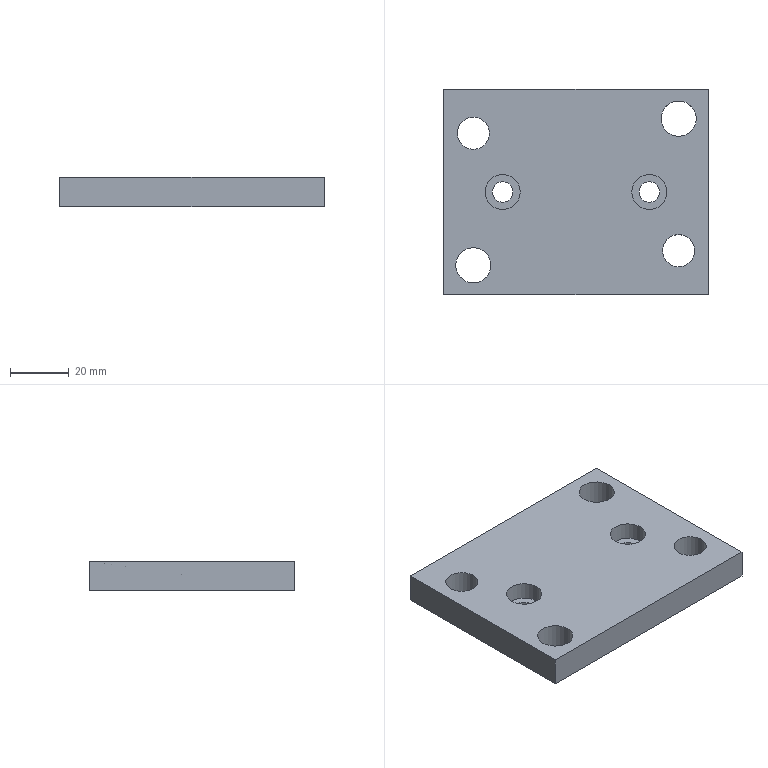Part | NX | features solid 2 | 1 solid | 16 faces | box 90 x 70 x 10 mm | volume 57172 mm3 | plane 8 | cylinder 8 | commonest cylinder face diameters 12 x4 7 x2 11 x2
STEP:
#1=CARTESIAN_POINT('',(594.,70.,60.));
#2=VERTEX_POINT('',#1);
#3=CARTESIAN_POINT('',(600.,70.,60.));
#4=DIRECTION('',(0.,0.,-1.));
#5=DIRECTION('',(-1.,0.,0.));
#6=AXIS2_PLACEMENT_3D('',#3,#4,#5);
#7=CIRCLE('',#6,6.);
#8=EDGE_CURVE('',#2,#2,#7,.F.);
#9=ORIENTED_EDGE('',*,*,#8,.F.);
#10=EDGE_LOOP('',(#9));
#11=FACE_BOUND('',#10,.T.);
#12=CARTESIAN_POINT('',(524.,20.,60.));
#13=VERTEX_POINT('',#12);
#14=CARTESIAN_POINT('',(530.,20.,60.));
#15=DIRECTION('',(0.,0.,-1.));
#16=DIRECTION('',(-1.,0.,0.));
#17=AXIS2_PLACEMENT_3D('',#14,#15,#16);
#18=CIRCLE('',#17,6.);
#19=EDGE_CURVE('',#13,#13,#18,.F.);
#20=ORIENTED_EDGE('',*,*,#19,.F.);
#21=EDGE_LOOP('',(#20));
#22=FACE_BOUND('',#21,.T.);
#23=CARTESIAN_POINT('',(584.,45.,60.));
#24=VERTEX_POINT('',#23);
#25=CARTESIAN_POINT('',(590.,45.,60.));
#26=DIRECTION('',(0.,0.,-1.));
#27=DIRECTION('',(-1.,0.,0.));
#28=AXIS2_PLACEMENT_3D('',#25,#26,#27);
#29=CIRCLE('',#28,6.);
#30=EDGE_CURVE('',#24,#24,#29,.T.);
#31=ORIENTED_EDGE('',*,*,#30,.T.);
#32=EDGE_LOOP('',(#31));
#33=FACE_BOUND('',#32,.T.);
#34=CARTESIAN_POINT('',(534.,45.,60.));
#35=VERTEX_POINT('',#34);
#36=CARTESIAN_POINT('',(540.,45.,60.));
#37=DIRECTION('',(0.,0.,-1.));
#38=DIRECTION('',(-1.,0.,0.));
#39=AXIS2_PLACEMENT_3D('',#36,#37,#38);
#40=CIRCLE('',#39,6.);
#41=EDGE_CURVE('',#35,#35,#40,.T.);
#42=ORIENTED_EDGE('',*,*,#41,.T.);
#43=EDGE_LOOP('',(#42));
#44=FACE_BOUND('',#43,.T.);
#45=CARTESIAN_POINT('',(610.,10.,60.));
#46=VERTEX_POINT('',#45);
#47=CARTESIAN_POINT('',(520.,10.,60.));
#48=VERTEX_POINT('',#47);
#49=CARTESIAN_POINT('',(610.,10.,60.));
#50=DIRECTION('',(-1.,0.,0.));
#51=VECTOR('',#50,1000.);
#52=LINE('',#49,#51);
#53=EDGE_CURVE('',#46,#48,#52,.T.);
#54=ORIENTED_EDGE('',*,*,#53,.F.);
#55=CARTESIAN_POINT('',(610.,80.,60.));
#56=VERTEX_POINT('',#55);
#57=CARTESIAN_POINT('',(610.,80.,60.));
#58=DIRECTION('',(0.,-1.,0.));
#59=VECTOR('',#58,1000.);
#60=LINE('',#57,#59);
#61=EDGE_CURVE('',#56,#46,#60,.T.);
#62=ORIENTED_EDGE('',*,*,#61,.F.);
#63=CARTESIAN_POINT('',(520.,80.,60.));
#64=VERTEX_POINT('',#63);
#65=CARTESIAN_POINT('',(520.,80.,60.));
#66=DIRECTION('',(1.,0.,0.));
#67=VECTOR('',#66,1000.);
#68=LINE('',#65,#67);
#69=EDGE_CURVE('',#64,#56,#68,.T.);
#70=ORIENTED_EDGE('',*,*,#69,.F.);
#71=CARTESIAN_POINT('',(520.,10.,60.));
#72=DIRECTION('',(0.,1.,0.));
#73=VECTOR('',#72,1000.);
#74=LINE('',#71,#73);
#75=EDGE_CURVE('',#48,#64,#74,.T.);
#76=ORIENTED_EDGE('',*,*,#75,.F.);
#77=EDGE_LOOP('',(#54,#62,#70,#76));
#78=FACE_BOUND('',#77,.T.);
#79=CARTESIAN_POINT('',(594.5,25.,60.));
#80=VERTEX_POINT('',#79);
#81=CARTESIAN_POINT('',(600.,25.,60.));
#82=DIRECTION('',(0.,0.,-1.));
#83=DIRECTION('',(-1.,0.,0.));
#84=AXIS2_PLACEMENT_3D('',#81,#82,#83);
#85=CIRCLE('',#84,5.5);
#86=EDGE_CURVE('',#80,#80,#85,.F.);
#87=ORIENTED_EDGE('',*,*,#86,.F.);
#88=EDGE_LOOP('',(#87));
#89=FACE_BOUND('',#88,.T.);
#90=CARTESIAN_POINT('',(524.5,65.,60.));
#91=VERTEX_POINT('',#90);
#92=CARTESIAN_POINT('',(530.,65.,60.));
#93=DIRECTION('',(0.,0.,-1.));
#94=DIRECTION('',(-1.,0.,0.));
#95=AXIS2_PLACEMENT_3D('',#92,#93,#94);
#96=CIRCLE('',#95,5.5);
#97=EDGE_CURVE('',#91,#91,#96,.F.);
#98=ORIENTED_EDGE('',*,*,#97,.F.);
#99=EDGE_LOOP('',(#98));
#100=FACE_BOUND('',#99,.T.);
#101=CARTESIAN_POINT('',(520.,10.,60.));
#102=DIRECTION('',(0.,0.,-1.));
#103=DIRECTION('',(-1.,0.,0.));
#104=AXIS2_PLACEMENT_3D('',#101,#102,#103);
#105=PLANE('',#104);
#106=ADVANCED_FACE('',(#11,#22,#33,#44,#78,#89,#100),#105,.F.);
#107=CARTESIAN_POINT('',(594.,70.,50.));
#108=VERTEX_POINT('',#107);
#109=CARTESIAN_POINT('',(600.,70.,50.));
#110=DIRECTION('',(0.,0.,-1.));
#111=DIRECTION('',(-1.,0.,0.));
#112=AXIS2_PLACEMENT_3D('',#109,#110,#111);
#113=CIRCLE('',#112,6.);
#114=EDGE_CURVE('',#108,#108,#113,.T.);
#115=ORIENTED_EDGE('',*,*,#114,.F.);
#116=EDGE_LOOP('',(#115));
#117=FACE_BOUND('',#116,.T.);
#118=CARTESIAN_POINT('',(524.,20.,50.));
#119=VERTEX_POINT('',#118);
#120=CARTESIAN_POINT('',(530.,20.,50.));
#121=DIRECTION('',(0.,0.,-1.));
#122=DIRECTION('',(-1.,0.,0.));
#123=AXIS2_PLACEMENT_3D('',#120,#121,#122);
#124=CIRCLE('',#123,6.);
#125=EDGE_CURVE('',#119,#119,#124,.T.);
#126=ORIENTED_EDGE('',*,*,#125,.F.);
#127=EDGE_LOOP('',(#126));
#128=FACE_BOUND('',#127,.T.);
#129=CARTESIAN_POINT('',(586.5,45.,50.));
#130=VERTEX_POINT('',#129);
#131=CARTESIAN_POINT('',(590.,45.,50.));
#132=DIRECTION('',(0.,0.,-1.));
#133=DIRECTION('',(-1.,0.,0.));
#134=AXIS2_PLACEMENT_3D('',#131,#132,#133);
#135=CIRCLE('',#134,3.5);
#136=EDGE_CURVE('',#130,#130,#135,.T.);
#137=ORIENTED_EDGE('',*,*,#136,.F.);
#138=EDGE_LOOP('',(#137));
#139=FACE_BOUND('',#138,.T.);
#140=CARTESIAN_POINT('',(536.5,45.,50.));
#141=VERTEX_POINT('',#140);
#142=CARTESIAN_POINT('',(540.,45.,50.));
#143=DIRECTION('',(0.,0.,-1.));
#144=DIRECTION('',(-1.,0.,0.));
#145=AXIS2_PLACEMENT_3D('',#142,#143,#144);
#146=CIRCLE('',#145,3.5);
#147=EDGE_CURVE('',#141,#141,#146,.T.);
#148=ORIENTED_EDGE('',*,*,#147,.F.);
#149=EDGE_LOOP('',(#148));
#150=FACE_BOUND('',#149,.T.);
#151=CARTESIAN_POINT('',(610.,10.,50.));
#152=VERTEX_POINT('',#151);
#153=CARTESIAN_POINT('',(520.,10.,50.));
#154=VERTEX_POINT('',#153);
#155=CARTESIAN_POINT('',(610.,10.,50.));
#156=DIRECTION('',(-1.,0.,0.));
#157=VECTOR('',#156,1000.);
#158=LINE('',#155,#157);
#159=EDGE_CURVE('',#152,#154,#158,.T.);
#160=ORIENTED_EDGE('',*,*,#159,.T.);
#161=CARTESIAN_POINT('',(520.,80.,50.));
#162=VERTEX_POINT('',#161);
#163=CARTESIAN_POINT('',(520.,10.,50.));
#164=DIRECTION('',(0.,1.,0.));
#165=VECTOR('',#164,1000.);
#166=LINE('',#163,#165);
#167=EDGE_CURVE('',#154,#162,#166,.T.);
#168=ORIENTED_EDGE('',*,*,#167,.T.);
#169=CARTESIAN_POINT('',(610.,80.,50.));
#170=VERTEX_POINT('',#169);
#171=CARTESIAN_POINT('',(520.,80.,50.));
#172=DIRECTION('',(1.,0.,0.));
#173=VECTOR('',#172,1000.);
#174=LINE('',#171,#173);
#175=EDGE_CURVE('',#162,#170,#174,.T.);
#176=ORIENTED_EDGE('',*,*,#175,.T.);
#177=CARTESIAN_POINT('',(610.,80.,50.));
#178=DIRECTION('',(0.,-1.,0.));
#179=VECTOR('',#178,1000.);
#180=LINE('',#177,#179);
#181=EDGE_CURVE('',#170,#152,#180,.T.);
#182=ORIENTED_EDGE('',*,*,#181,.T.);
#183=EDGE_LOOP('',(#160,#168,#176,#182));
#184=FACE_BOUND('',#183,.T.);
#185=CARTESIAN_POINT('',(594.5,25.,50.));
#186=VERTEX_POINT('',#185);
#187=CARTESIAN_POINT('',(600.,25.,50.));
#188=DIRECTION('',(0.,0.,-1.));
#189=DIRECTION('',(-1.,0.,0.));
#190=AXIS2_PLACEMENT_3D('',#187,#188,#189);
#191=CIRCLE('',#190,5.5);
#192=EDGE_CURVE('',#186,#186,#191,.T.);
#193=ORIENTED_EDGE('',*,*,#192,.F.);
#194=EDGE_LOOP('',(#193));
#195=FACE_BOUND('',#194,.T.);
#196=CARTESIAN_POINT('',(524.5,65.,50.));
#197=VERTEX_POINT('',#196);
#198=CARTESIAN_POINT('',(530.,65.,50.));
#199=DIRECTION('',(0.,0.,-1.));
#200=DIRECTION('',(-1.,0.,0.));
#201=AXIS2_PLACEMENT_3D('',#198,#199,#200);
#202=CIRCLE('',#201,5.5);
#203=EDGE_CURVE('',#197,#197,#202,.T.);
#204=ORIENTED_EDGE('',*,*,#203,.F.);
#205=EDGE_LOOP('',(#204));
#206=FACE_BOUND('',#205,.T.);
#207=CARTESIAN_POINT('',(520.,10.,50.));
#208=DIRECTION('',(0.,0.,-1.));
#209=DIRECTION('',(-1.,0.,0.));
#210=AXIS2_PLACEMENT_3D('',#207,#208,#209);
#211=PLANE('',#210);
#212=ADVANCED_FACE('',(#117,#128,#139,#150,#184,#195,#206),#211,.T.);
#213=ORIENTED_EDGE('',*,*,#159,.F.);
#214=CARTESIAN_POINT('',(610.,10.,60.));
#215=DIRECTION('',(0.,0.,-1.));
#216=VECTOR('',#215,1000.);
#217=LINE('',#214,#216);
#218=EDGE_CURVE('',#46,#152,#217,.T.);
#219=ORIENTED_EDGE('',*,*,#218,.F.);
#220=ORIENTED_EDGE('',*,*,#53,.T.);
#221=CARTESIAN_POINT('',(520.,10.,60.));
#222=DIRECTION('',(0.,0.,-1.));
#223=VECTOR('',#222,1000.);
#224=LINE('',#221,#223);
#225=EDGE_CURVE('',#48,#154,#224,.T.);
#226=ORIENTED_EDGE('',*,*,#225,.T.);
#227=EDGE_LOOP('',(#213,#219,#220,#226));
#228=FACE_BOUND('',#227,.T.);
#229=CARTESIAN_POINT('',(610.,10.,60.));
#230=DIRECTION('',(0.,-1.,0.));
#231=DIRECTION('',(0.,0.,-1.));
#232=AXIS2_PLACEMENT_3D('',#229,#230,#231);
#233=PLANE('',#232);
#234=ADVANCED_FACE('',(#228),#233,.T.);
#235=ORIENTED_EDGE('',*,*,#167,.F.);
#236=ORIENTED_EDGE('',*,*,#225,.F.);
#237=ORIENTED_EDGE('',*,*,#75,.T.);
#238=CARTESIAN_POINT('',(520.,80.,60.));
#239=DIRECTION('',(0.,0.,-1.));
#240=VECTOR('',#239,1000.);
#241=LINE('',#238,#240);
#242=EDGE_CURVE('',#64,#162,#241,.T.);
#243=ORIENTED_EDGE('',*,*,#242,.T.);
#244=EDGE_LOOP('',(#235,#236,#237,#243));
#245=FACE_BOUND('',#244,.T.);
#246=CARTESIAN_POINT('',(520.,10.,60.));
#247=DIRECTION('',(-1.,0.,0.));
#248=DIRECTION('',(0.,0.,1.));
#249=AXIS2_PLACEMENT_3D('',#246,#247,#248);
#250=PLANE('',#249);
#251=ADVANCED_FACE('',(#245),#250,.T.);
#252=ORIENTED_EDGE('',*,*,#175,.F.);
#253=ORIENTED_EDGE('',*,*,#242,.F.);
#254=ORIENTED_EDGE('',*,*,#69,.T.);
#255=CARTESIAN_POINT('',(610.,80.,60.));
#256=DIRECTION('',(0.,0.,-1.));
#257=VECTOR('',#256,1000.);
#258=LINE('',#255,#257);
#259=EDGE_CURVE('',#56,#170,#258,.T.);
#260=ORIENTED_EDGE('',*,*,#259,.T.);
#261=EDGE_LOOP('',(#252,#253,#254,#260));
#262=FACE_BOUND('',#261,.T.);
#263=CARTESIAN_POINT('',(520.,80.,60.));
#264=DIRECTION('',(0.,1.,0.));
#265=DIRECTION('',(0.,0.,1.));
#266=AXIS2_PLACEMENT_3D('',#263,#264,#265);
#267=PLANE('',#266);
#268=ADVANCED_FACE('',(#262),#267,.T.);
#269=ORIENTED_EDGE('',*,*,#181,.F.);
#270=ORIENTED_EDGE('',*,*,#259,.F.);
#271=ORIENTED_EDGE('',*,*,#61,.T.);
#272=ORIENTED_EDGE('',*,*,#218,.T.);
#273=EDGE_LOOP('',(#269,#270,#271,#272));
#274=FACE_BOUND('',#273,.T.);
#275=CARTESIAN_POINT('',(610.,80.,60.));
#276=DIRECTION('',(1.,0.,0.));
#277=DIRECTION('',(0.,0.,-1.));
#278=AXIS2_PLACEMENT_3D('',#275,#276,#277);
#279=PLANE('',#278);
#280=ADVANCED_FACE('',(#274),#279,.T.);
#281=ORIENTED_EDGE('',*,*,#147,.T.);
#282=EDGE_LOOP('',(#281));
#283=FACE_BOUND('',#282,.T.);
#284=CARTESIAN_POINT('',(536.5,45.,54.));
#285=VERTEX_POINT('',#284);
#286=CARTESIAN_POINT('',(540.,45.,54.));
#287=DIRECTION('',(0.,0.,-1.));
#288=DIRECTION('',(-1.,0.,0.));
#289=AXIS2_PLACEMENT_3D('',#286,#287,#288);
#290=CIRCLE('',#289,3.5);
#291=EDGE_CURVE('',#285,#285,#290,.T.);
#292=ORIENTED_EDGE('',*,*,#291,.F.);
#293=EDGE_LOOP('',(#292));
#294=FACE_BOUND('',#293,.T.);
#295=CARTESIAN_POINT('',(540.,45.,10.));
#296=DIRECTION('',(0.,0.,-1.));
#297=DIRECTION('',(-1.,0.,0.));
#298=AXIS2_PLACEMENT_3D('',#295,#296,#297);
#299=CYLINDRICAL_SURFACE('',#298,3.5);
#300=ADVANCED_FACE('',(#283,#294),#299,.F.);
#301=ORIENTED_EDGE('',*,*,#291,.T.);
#302=EDGE_LOOP('',(#301));
#303=FACE_BOUND('',#302,.T.);
#304=CARTESIAN_POINT('',(534.,45.,54.));
#305=VERTEX_POINT('',#304);
#306=CARTESIAN_POINT('',(540.,45.,54.));
#307=DIRECTION('',(0.,0.,-1.));
#308=DIRECTION('',(-1.,0.,0.));
#309=AXIS2_PLACEMENT_3D('',#306,#307,#308);
#310=CIRCLE('',#309,6.);
#311=EDGE_CURVE('',#305,#305,#310,.T.);
#312=ORIENTED_EDGE('',*,*,#311,.F.);
#313=EDGE_LOOP('',(#312));
#314=FACE_BOUND('',#313,.T.);
#315=CARTESIAN_POINT('',(540.,45.,54.));
#316=DIRECTION('',(0.,0.,-1.));
#317=DIRECTION('',(-1.,0.,0.));
#318=AXIS2_PLACEMENT_3D('',#315,#316,#317);
#319=PLANE('',#318);
#320=ADVANCED_FACE('',(#303,#314),#319,.F.);
#321=ORIENTED_EDGE('',*,*,#311,.T.);
#322=EDGE_LOOP('',(#321));
#323=FACE_BOUND('',#322,.T.);
#324=ORIENTED_EDGE('',*,*,#41,.F.);
#325=EDGE_LOOP('',(#324));
#326=FACE_BOUND('',#325,.T.);
#327=CARTESIAN_POINT('',(540.,45.,60.));
#328=DIRECTION('',(0.,0.,-1.));
#329=DIRECTION('',(-1.,0.,0.));
#330=AXIS2_PLACEMENT_3D('',#327,#328,#329);
#331=CYLINDRICAL_SURFACE('',#330,6.);
#332=ADVANCED_FACE('',(#323,#326),#331,.F.);
#333=ORIENTED_EDGE('',*,*,#136,.T.);
#334=EDGE_LOOP('',(#333));
#335=FACE_BOUND('',#334,.T.);
#336=CARTESIAN_POINT('',(586.5,45.,54.));
#337=VERTEX_POINT('',#336);
#338=CARTESIAN_POINT('',(590.,45.,54.));
#339=DIRECTION('',(0.,0.,-1.));
#340=DIRECTION('',(-1.,0.,0.));
#341=AXIS2_PLACEMENT_3D('',#338,#339,#340);
#342=CIRCLE('',#341,3.5);
#343=EDGE_CURVE('',#337,#337,#342,.T.);
#344=ORIENTED_EDGE('',*,*,#343,.F.);
#345=EDGE_LOOP('',(#344));
#346=FACE_BOUND('',#345,.T.);
#347=CARTESIAN_POINT('',(590.,45.,10.));
#348=DIRECTION('',(0.,0.,-1.));
#349=DIRECTION('',(-1.,0.,0.));
#350=AXIS2_PLACEMENT_3D('',#347,#348,#349);
#351=CYLINDRICAL_SURFACE('',#350,3.5);
#352=ADVANCED_FACE('',(#335,#346),#351,.F.);
#353=ORIENTED_EDGE('',*,*,#343,.T.);
#354=EDGE_LOOP('',(#353));
#355=FACE_BOUND('',#354,.T.);
#356=CARTESIAN_POINT('',(584.,45.,54.));
#357=VERTEX_POINT('',#356);
#358=CARTESIAN_POINT('',(590.,45.,54.));
#359=DIRECTION('',(0.,0.,-1.));
#360=DIRECTION('',(-1.,0.,0.));
#361=AXIS2_PLACEMENT_3D('',#358,#359,#360);
#362=CIRCLE('',#361,6.);
#363=EDGE_CURVE('',#357,#357,#362,.T.);
#364=ORIENTED_EDGE('',*,*,#363,.F.);
#365=EDGE_LOOP('',(#364));
#366=FACE_BOUND('',#365,.T.);
#367=CARTESIAN_POINT('',(590.,45.,54.));
#368=DIRECTION('',(0.,0.,-1.));
#369=DIRECTION('',(-1.,0.,0.));
#370=AXIS2_PLACEMENT_3D('',#367,#368,#369);
#371=PLANE('',#370);
#372=ADVANCED_FACE('',(#355,#366),#371,.F.);
#373=ORIENTED_EDGE('',*,*,#363,.T.);
#374=EDGE_LOOP('',(#373));
#375=FACE_BOUND('',#374,.T.);
#376=ORIENTED_EDGE('',*,*,#30,.F.);
#377=EDGE_LOOP('',(#376));
#378=FACE_BOUND('',#377,.T.);
#379=CARTESIAN_POINT('',(590.,45.,60.));
#380=DIRECTION('',(0.,0.,-1.));
#381=DIRECTION('',(-1.,0.,0.));
#382=AXIS2_PLACEMENT_3D('',#379,#380,#381);
#383=CYLINDRICAL_SURFACE('',#382,6.);
#384=ADVANCED_FACE('',(#375,#378),#383,.F.);
#385=ORIENTED_EDGE('',*,*,#125,.T.);
#386=EDGE_LOOP('',(#385));
#387=FACE_BOUND('',#386,.T.);
#388=ORIENTED_EDGE('',*,*,#19,.T.);
#389=EDGE_LOOP('',(#388));
#390=FACE_BOUND('',#389,.T.);
#391=CARTESIAN_POINT('',(530.,20.,50.));
#392=DIRECTION('',(0.,0.,1.));
#393=DIRECTION('',(1.,0.,0.));
#394=AXIS2_PLACEMENT_3D('',#391,#392,#393);
#395=CYLINDRICAL_SURFACE('',#394,6.);
#396=ADVANCED_FACE('',(#387,#390),#395,.F.);
#397=ORIENTED_EDGE('',*,*,#192,.T.);
#398=EDGE_LOOP('',(#397));
#399=FACE_BOUND('',#398,.T.);
#400=ORIENTED_EDGE('',*,*,#86,.T.);
#401=EDGE_LOOP('',(#400));
#402=FACE_BOUND('',#401,.T.);
#403=CARTESIAN_POINT('',(600.,25.,50.));
#404=DIRECTION('',(0.,0.,1.));
#405=DIRECTION('',(1.,0.,0.));
#406=AXIS2_PLACEMENT_3D('',#403,#404,#405);
#407=CYLINDRICAL_SURFACE('',#406,5.5);
#408=ADVANCED_FACE('',(#399,#402),#407,.F.);
#409=ORIENTED_EDGE('',*,*,#114,.T.);
#410=EDGE_LOOP('',(#409));
#411=FACE_BOUND('',#410,.T.);
#412=ORIENTED_EDGE('',*,*,#8,.T.);
#413=EDGE_LOOP('',(#412));
#414=FACE_BOUND('',#413,.T.);
#415=CARTESIAN_POINT('',(600.,70.,50.));
#416=DIRECTION('',(0.,0.,1.));
#417=DIRECTION('',(1.,0.,0.));
#418=AXIS2_PLACEMENT_3D('',#415,#416,#417);
#419=CYLINDRICAL_SURFACE('',#418,6.);
#420=ADVANCED_FACE('',(#411,#414),#419,.F.);
#421=ORIENTED_EDGE('',*,*,#203,.T.);
#422=EDGE_LOOP('',(#421));
#423=FACE_BOUND('',#422,.T.);
#424=ORIENTED_EDGE('',*,*,#97,.T.);
#425=EDGE_LOOP('',(#424));
#426=FACE_BOUND('',#425,.T.);
#427=CARTESIAN_POINT('',(530.,65.,50.));
#428=DIRECTION('',(0.,0.,1.));
#429=DIRECTION('',(1.,0.,0.));
#430=AXIS2_PLACEMENT_3D('',#427,#428,#429);
#431=CYLINDRICAL_SURFACE('',#430,5.5);
#432=ADVANCED_FACE('',(#423,#426),#431,.F.);
#433=CLOSED_SHELL('',(#106,#212,#234,#251,#268,#280,#300,#320,#332,#352,#372,#384,#396,#408,#420,#432));
#434=MANIFOLD_SOLID_BREP('',#433);
#435=(LENGTH_UNIT()NAMED_UNIT(*)SI_UNIT(.MILLI.,.METRE.));
#436=UNCERTAINTY_MEASURE_WITH_UNIT(LENGTH_MEASURE(0.00001),#435,'','');
#437=(NAMED_UNIT(*)PLANE_ANGLE_UNIT()SI_UNIT($,.RADIAN.));
#438=(NAMED_UNIT(*)SI_UNIT($,.STERADIAN.)SOLID_ANGLE_UNIT());
#439=(GEOMETRIC_REPRESENTATION_CONTEXT(3)GLOBAL_UNCERTAINTY_ASSIGNED_CONTEXT((#436))GLOBAL_UNIT_ASSIGNED_CONTEXT((#435,#437,#438))REPRESENTATION_CONTEXT('',''));
#440=ADVANCED_BREP_SHAPE_REPRESENTATION('',(#434),#439);